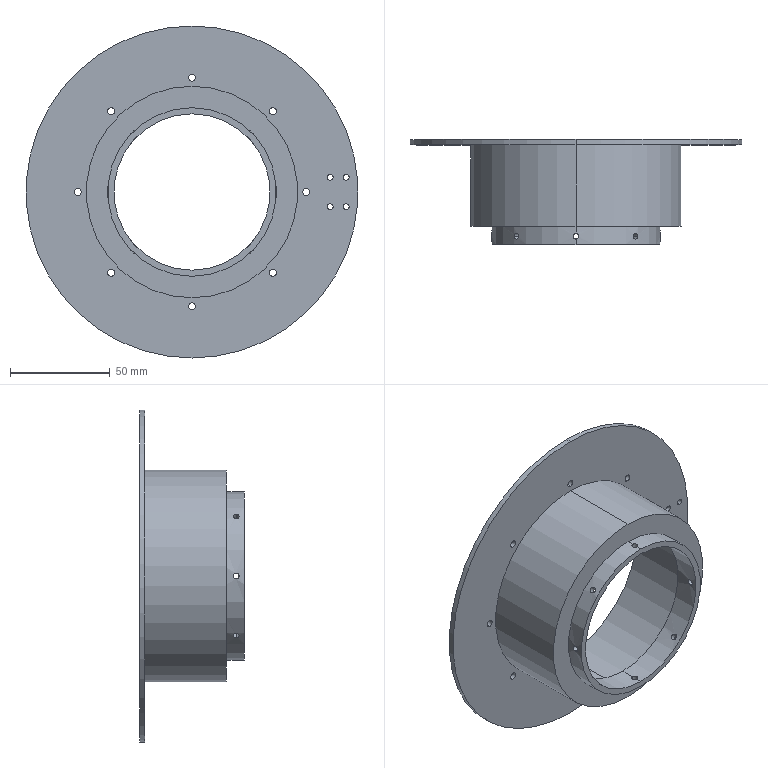Part | SolidWorks | features SavedExtBody 1 | 1 solid | 55 faces | box 166.652 x 52.651 x 166.652 mm | volume 97043 mm3 | cylinder 50 | plane 5 | commonest cylinder face diameters 3 x24 3.5 x16 78.435 x2 84.561 x2 99.754 x2 106.126 x2